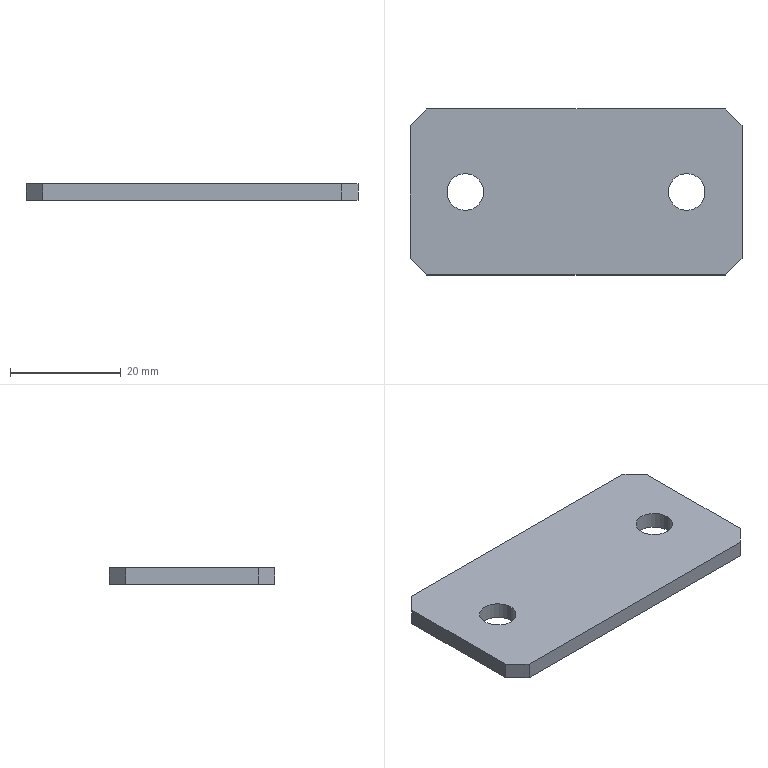Part | STEP file | HXGR200008-05-15 | 1 solid | 14 faces | box 60 x 30 x 3 mm | volume 5141 mm3 | plane 10 | cylinder 4 | commonest cylinder face diameters 6.6 x4
STEP:
#1=CARTESIAN_POINT('',(-23.3,0.,-3.));
#2=VERTEX_POINT('',#1);
#3=CARTESIAN_POINT('',(-16.7,0.,-3.));
#4=VERTEX_POINT('',#3);
#5=CARTESIAN_POINT('',(-20.,0.,-3.));
#6=DIRECTION('',(0.,0.,1.));
#7=DIRECTION('',(1.,0.,0.));
#8=AXIS2_PLACEMENT_3D('',#5,#6,#7);
#9=CIRCLE('',#8,3.3);
#10=EDGE_CURVE('',#2,#4,#9,.T.);
#11=ORIENTED_EDGE('',*,*,#10,.F.);
#12=CARTESIAN_POINT('',(-23.3,0.,0.));
#13=VERTEX_POINT('',#12);
#14=CARTESIAN_POINT('',(-23.3,0.,0.));
#15=DIRECTION('',(0.,0.,1.));
#16=VECTOR('',#15,1000.);
#17=LINE('',#14,#16);
#18=EDGE_CURVE('',#2,#13,#17,.T.);
#19=ORIENTED_EDGE('',*,*,#18,.T.);
#20=CARTESIAN_POINT('',(-16.7,0.,0.));
#21=VERTEX_POINT('',#20);
#22=CARTESIAN_POINT('',(-20.,0.,0.));
#23=DIRECTION('',(0.,0.,1.));
#24=DIRECTION('',(1.,0.,0.));
#25=AXIS2_PLACEMENT_3D('',#22,#23,#24);
#26=CIRCLE('',#25,3.3);
#27=EDGE_CURVE('',#13,#21,#26,.T.);
#28=ORIENTED_EDGE('',*,*,#27,.T.);
#29=CARTESIAN_POINT('',(-16.7,0.,0.));
#30=DIRECTION('',(0.,0.,1.));
#31=VECTOR('',#30,1000.);
#32=LINE('',#29,#31);
#33=EDGE_CURVE('',#4,#21,#32,.T.);
#34=ORIENTED_EDGE('',*,*,#33,.F.);
#35=EDGE_LOOP('',(#11,#19,#28,#34));
#36=FACE_OUTER_BOUND('',#35,.T.);
#37=CARTESIAN_POINT('',(-20.,0.,0.));
#38=DIRECTION('',(0.,0.,1.));
#39=DIRECTION('',(1.,0.,0.));
#40=AXIS2_PLACEMENT_3D('',#37,#38,#39);
#41=CYLINDRICAL_SURFACE('',#40,3.3);
#42=ADVANCED_FACE('',(#36),#41,.F.);
#43=CARTESIAN_POINT('',(16.7,0.,-3.));
#44=VERTEX_POINT('',#43);
#45=CARTESIAN_POINT('',(23.3,0.,-3.));
#46=VERTEX_POINT('',#45);
#47=CARTESIAN_POINT('',(20.,0.,-3.));
#48=DIRECTION('',(0.,0.,1.));
#49=DIRECTION('',(1.,0.,0.));
#50=AXIS2_PLACEMENT_3D('',#47,#48,#49);
#51=CIRCLE('',#50,3.3);
#52=EDGE_CURVE('',#44,#46,#51,.T.);
#53=ORIENTED_EDGE('',*,*,#52,.F.);
#54=CARTESIAN_POINT('',(16.7,0.,0.));
#55=VERTEX_POINT('',#54);
#56=CARTESIAN_POINT('',(16.7,0.,0.));
#57=DIRECTION('',(0.,0.,1.));
#58=VECTOR('',#57,1000.);
#59=LINE('',#56,#58);
#60=EDGE_CURVE('',#44,#55,#59,.T.);
#61=ORIENTED_EDGE('',*,*,#60,.T.);
#62=CARTESIAN_POINT('',(23.3,0.,0.));
#63=VERTEX_POINT('',#62);
#64=CARTESIAN_POINT('',(20.,0.,0.));
#65=DIRECTION('',(0.,0.,1.));
#66=DIRECTION('',(1.,0.,0.));
#67=AXIS2_PLACEMENT_3D('',#64,#65,#66);
#68=CIRCLE('',#67,3.3);
#69=EDGE_CURVE('',#55,#63,#68,.T.);
#70=ORIENTED_EDGE('',*,*,#69,.T.);
#71=CARTESIAN_POINT('',(23.3,0.,0.));
#72=DIRECTION('',(0.,0.,1.));
#73=VECTOR('',#72,1000.);
#74=LINE('',#71,#73);
#75=EDGE_CURVE('',#46,#63,#74,.T.);
#76=ORIENTED_EDGE('',*,*,#75,.F.);
#77=EDGE_LOOP('',(#53,#61,#70,#76));
#78=FACE_OUTER_BOUND('',#77,.T.);
#79=CARTESIAN_POINT('',(20.,0.,0.));
#80=DIRECTION('',(0.,0.,1.));
#81=DIRECTION('',(1.,0.,0.));
#82=AXIS2_PLACEMENT_3D('',#79,#80,#81);
#83=CYLINDRICAL_SURFACE('',#82,3.3);
#84=ADVANCED_FACE('',(#78),#83,.F.);
#85=CARTESIAN_POINT('',(30.,-12.,-3.));
#86=VERTEX_POINT('',#85);
#87=CARTESIAN_POINT('',(30.,12.,-3.));
#88=VERTEX_POINT('',#87);
#89=CARTESIAN_POINT('',(30.,15.,-3.));
#90=DIRECTION('',(0.,1.,0.));
#91=VECTOR('',#90,1000.);
#92=LINE('',#89,#91);
#93=EDGE_CURVE('',#86,#88,#92,.T.);
#94=ORIENTED_EDGE('',*,*,#93,.T.);
#95=CARTESIAN_POINT('',(30.,12.,0.));
#96=VERTEX_POINT('',#95);
#97=CARTESIAN_POINT('',(30.,12.,-3.));
#98=DIRECTION('',(0.,0.,1.));
#99=VECTOR('',#98,1000.);
#100=LINE('',#97,#99);
#101=EDGE_CURVE('',#88,#96,#100,.T.);
#102=ORIENTED_EDGE('',*,*,#101,.T.);
#103=CARTESIAN_POINT('',(30.,-12.,0.));
#104=VERTEX_POINT('',#103);
#105=CARTESIAN_POINT('',(30.,15.,0.));
#106=DIRECTION('',(0.,1.,0.));
#107=VECTOR('',#106,1000.);
#108=LINE('',#105,#107);
#109=EDGE_CURVE('',#104,#96,#108,.T.);
#110=ORIENTED_EDGE('',*,*,#109,.F.);
#111=CARTESIAN_POINT('',(30.,-12.,-3.));
#112=DIRECTION('',(0.,0.,-1.));
#113=VECTOR('',#112,1000.);
#114=LINE('',#111,#113);
#115=EDGE_CURVE('',#104,#86,#114,.T.);
#116=ORIENTED_EDGE('',*,*,#115,.T.);
#117=EDGE_LOOP('',(#94,#102,#110,#116));
#118=FACE_OUTER_BOUND('',#117,.T.);
#119=CARTESIAN_POINT('',(30.,15.,-3.));
#120=DIRECTION('',(1.,0.,0.));
#121=DIRECTION('',(0.,1.,0.));
#122=AXIS2_PLACEMENT_3D('',#119,#120,#121);
#123=PLANE('',#122);
#124=ADVANCED_FACE('',(#118),#123,.T.);
#125=CARTESIAN_POINT('',(-27.,-15.,-3.));
#126=VERTEX_POINT('',#125);
#127=CARTESIAN_POINT('',(27.,-15.,-3.));
#128=VERTEX_POINT('',#127);
#129=CARTESIAN_POINT('',(-30.,-15.,-3.));
#130=DIRECTION('',(1.,0.,0.));
#131=VECTOR('',#130,1000.);
#132=LINE('',#129,#131);
#133=EDGE_CURVE('',#126,#128,#132,.T.);
#134=ORIENTED_EDGE('',*,*,#133,.T.);
#135=CARTESIAN_POINT('',(27.,-15.,0.));
#136=VERTEX_POINT('',#135);
#137=CARTESIAN_POINT('',(27.,-15.,-3.));
#138=DIRECTION('',(0.,0.,1.));
#139=VECTOR('',#138,1000.);
#140=LINE('',#137,#139);
#141=EDGE_CURVE('',#128,#136,#140,.T.);
#142=ORIENTED_EDGE('',*,*,#141,.T.);
#143=CARTESIAN_POINT('',(-27.,-15.,0.));
#144=VERTEX_POINT('',#143);
#145=CARTESIAN_POINT('',(-30.,-15.,0.));
#146=DIRECTION('',(1.,0.,0.));
#147=VECTOR('',#146,1000.);
#148=LINE('',#145,#147);
#149=EDGE_CURVE('',#144,#136,#148,.T.);
#150=ORIENTED_EDGE('',*,*,#149,.F.);
#151=CARTESIAN_POINT('',(-27.,-15.,-3.));
#152=DIRECTION('',(0.,0.,-1.));
#153=VECTOR('',#152,1000.);
#154=LINE('',#151,#153);
#155=EDGE_CURVE('',#144,#126,#154,.T.);
#156=ORIENTED_EDGE('',*,*,#155,.T.);
#157=EDGE_LOOP('',(#134,#142,#150,#156));
#158=FACE_OUTER_BOUND('',#157,.T.);
#159=CARTESIAN_POINT('',(-30.,-15.,-3.));
#160=DIRECTION('',(0.,-1.,0.));
#161=DIRECTION('',(0.,0.,-1.));
#162=AXIS2_PLACEMENT_3D('',#159,#160,#161);
#163=PLANE('',#162);
#164=ADVANCED_FACE('',(#158),#163,.T.);
#165=CARTESIAN_POINT('',(-30.,12.,0.));
#166=VERTEX_POINT('',#165);
#167=CARTESIAN_POINT('',(-30.,-12.,0.));
#168=VERTEX_POINT('',#167);
#169=CARTESIAN_POINT('',(-30.,15.,0.));
#170=DIRECTION('',(0.,-1.,0.));
#171=VECTOR('',#170,1000.);
#172=LINE('',#169,#171);
#173=EDGE_CURVE('',#166,#168,#172,.T.);
#174=ORIENTED_EDGE('',*,*,#173,.F.);
#175=CARTESIAN_POINT('',(-30.,12.,-3.));
#176=VERTEX_POINT('',#175);
#177=CARTESIAN_POINT('',(-30.,12.,-3.));
#178=DIRECTION('',(0.,0.,-1.));
#179=VECTOR('',#178,1000.);
#180=LINE('',#177,#179);
#181=EDGE_CURVE('',#166,#176,#180,.T.);
#182=ORIENTED_EDGE('',*,*,#181,.T.);
#183=CARTESIAN_POINT('',(-30.,-12.,-3.));
#184=VERTEX_POINT('',#183);
#185=CARTESIAN_POINT('',(-30.,15.,-3.));
#186=DIRECTION('',(0.,-1.,0.));
#187=VECTOR('',#186,1000.);
#188=LINE('',#185,#187);
#189=EDGE_CURVE('',#176,#184,#188,.T.);
#190=ORIENTED_EDGE('',*,*,#189,.T.);
#191=CARTESIAN_POINT('',(-30.,-12.,-3.));
#192=DIRECTION('',(0.,0.,1.));
#193=VECTOR('',#192,1000.);
#194=LINE('',#191,#193);
#195=EDGE_CURVE('',#184,#168,#194,.T.);
#196=ORIENTED_EDGE('',*,*,#195,.T.);
#197=EDGE_LOOP('',(#174,#182,#190,#196));
#198=FACE_OUTER_BOUND('',#197,.T.);
#199=CARTESIAN_POINT('',(-30.,15.,-3.));
#200=DIRECTION('',(-1.,0.,0.));
#201=DIRECTION('',(0.,0.,1.));
#202=AXIS2_PLACEMENT_3D('',#199,#200,#201);
#203=PLANE('',#202);
#204=ADVANCED_FACE('',(#198),#203,.T.);
#205=CARTESIAN_POINT('',(27.,15.,-3.));
#206=VERTEX_POINT('',#205);
#207=CARTESIAN_POINT('',(-27.,15.,-3.));
#208=VERTEX_POINT('',#207);
#209=CARTESIAN_POINT('',(-30.,15.,-3.));
#210=DIRECTION('',(-1.,0.,0.));
#211=VECTOR('',#210,1000.);
#212=LINE('',#209,#211);
#213=EDGE_CURVE('',#206,#208,#212,.T.);
#214=ORIENTED_EDGE('',*,*,#213,.T.);
#215=CARTESIAN_POINT('',(-27.,15.,0.));
#216=VERTEX_POINT('',#215);
#217=CARTESIAN_POINT('',(-27.,15.,-3.));
#218=DIRECTION('',(0.,0.,1.));
#219=VECTOR('',#218,1000.);
#220=LINE('',#217,#219);
#221=EDGE_CURVE('',#208,#216,#220,.T.);
#222=ORIENTED_EDGE('',*,*,#221,.T.);
#223=CARTESIAN_POINT('',(27.,15.,0.));
#224=VERTEX_POINT('',#223);
#225=CARTESIAN_POINT('',(-30.,15.,0.));
#226=DIRECTION('',(-1.,0.,0.));
#227=VECTOR('',#226,1000.);
#228=LINE('',#225,#227);
#229=EDGE_CURVE('',#224,#216,#228,.T.);
#230=ORIENTED_EDGE('',*,*,#229,.F.);
#231=CARTESIAN_POINT('',(27.,15.,-3.));
#232=DIRECTION('',(0.,0.,-1.));
#233=VECTOR('',#232,1000.);
#234=LINE('',#231,#233);
#235=EDGE_CURVE('',#224,#206,#234,.T.);
#236=ORIENTED_EDGE('',*,*,#235,.T.);
#237=EDGE_LOOP('',(#214,#222,#230,#236));
#238=FACE_OUTER_BOUND('',#237,.T.);
#239=CARTESIAN_POINT('',(-30.,15.,-3.));
#240=DIRECTION('',(0.,1.,0.));
#241=DIRECTION('',(0.,0.,1.));
#242=AXIS2_PLACEMENT_3D('',#239,#240,#241);
#243=PLANE('',#242);
#244=ADVANCED_FACE('',(#238),#243,.T.);
#245=CARTESIAN_POINT('',(-20.,0.,-3.));
#246=DIRECTION('',(0.,0.,1.));
#247=DIRECTION('',(1.,0.,0.));
#248=AXIS2_PLACEMENT_3D('',#245,#246,#247);
#249=CIRCLE('',#248,3.3);
#250=EDGE_CURVE('',#4,#2,#249,.T.);
#251=ORIENTED_EDGE('',*,*,#250,.T.);
#252=ORIENTED_EDGE('',*,*,#10,.T.);
#253=EDGE_LOOP('',(#251,#252));
#254=FACE_BOUND('',#253,.T.);
#255=CARTESIAN_POINT('',(20.,0.,-3.));
#256=DIRECTION('',(0.,0.,1.));
#257=DIRECTION('',(1.,0.,0.));
#258=AXIS2_PLACEMENT_3D('',#255,#256,#257);
#259=CIRCLE('',#258,3.3);
#260=EDGE_CURVE('',#46,#44,#259,.T.);
#261=ORIENTED_EDGE('',*,*,#260,.T.);
#262=ORIENTED_EDGE('',*,*,#52,.T.);
#263=EDGE_LOOP('',(#261,#262));
#264=FACE_BOUND('',#263,.T.);
#265=ORIENTED_EDGE('',*,*,#189,.F.);
#266=CARTESIAN_POINT('',(-27.,15.,-3.));
#267=DIRECTION('',(0.7071,0.7071,0.));
#268=VECTOR('',#267,1000.);
#269=LINE('',#266,#268);
#270=EDGE_CURVE('',#176,#208,#269,.T.);
#271=ORIENTED_EDGE('',*,*,#270,.T.);
#272=ORIENTED_EDGE('',*,*,#213,.F.);
#273=CARTESIAN_POINT('',(30.,12.,-3.));
#274=DIRECTION('',(0.7071,-0.7071,0.));
#275=VECTOR('',#274,1000.);
#276=LINE('',#273,#275);
#277=EDGE_CURVE('',#206,#88,#276,.T.);
#278=ORIENTED_EDGE('',*,*,#277,.T.);
#279=ORIENTED_EDGE('',*,*,#93,.F.);
#280=CARTESIAN_POINT('',(27.,-15.,-3.));
#281=DIRECTION('',(-0.7071,-0.7071,0.));
#282=VECTOR('',#281,1000.);
#283=LINE('',#280,#282);
#284=EDGE_CURVE('',#86,#128,#283,.T.);
#285=ORIENTED_EDGE('',*,*,#284,.T.);
#286=ORIENTED_EDGE('',*,*,#133,.F.);
#287=CARTESIAN_POINT('',(-30.,-12.,-3.));
#288=DIRECTION('',(-0.7071,0.7071,0.));
#289=VECTOR('',#288,1000.);
#290=LINE('',#287,#289);
#291=EDGE_CURVE('',#126,#184,#290,.T.);
#292=ORIENTED_EDGE('',*,*,#291,.T.);
#293=EDGE_LOOP('',(#265,#271,#272,#278,#279,#285,#286,#292));
#294=FACE_OUTER_BOUND('',#293,.T.);
#295=CARTESIAN_POINT('',(0.,0.,-3.));
#296=DIRECTION('',(0.,0.,1.));
#297=DIRECTION('',(1.,0.,0.));
#298=AXIS2_PLACEMENT_3D('',#295,#296,#297);
#299=PLANE('',#298);
#300=ADVANCED_FACE('',(#254,#264,#294),#299,.F.);
#301=CARTESIAN_POINT('',(-20.,0.,0.));
#302=DIRECTION('',(0.,0.,1.));
#303=DIRECTION('',(1.,0.,0.));
#304=AXIS2_PLACEMENT_3D('',#301,#302,#303);
#305=CIRCLE('',#304,3.3);
#306=EDGE_CURVE('',#21,#13,#305,.T.);
#307=ORIENTED_EDGE('',*,*,#306,.F.);
#308=ORIENTED_EDGE('',*,*,#27,.F.);
#309=EDGE_LOOP('',(#307,#308));
#310=FACE_BOUND('',#309,.T.);
#311=CARTESIAN_POINT('',(20.,0.,0.));
#312=DIRECTION('',(0.,0.,1.));
#313=DIRECTION('',(1.,0.,0.));
#314=AXIS2_PLACEMENT_3D('',#311,#312,#313);
#315=CIRCLE('',#314,3.3);
#316=EDGE_CURVE('',#63,#55,#315,.T.);
#317=ORIENTED_EDGE('',*,*,#316,.F.);
#318=ORIENTED_EDGE('',*,*,#69,.F.);
#319=EDGE_LOOP('',(#317,#318));
#320=FACE_BOUND('',#319,.T.);
#321=ORIENTED_EDGE('',*,*,#229,.T.);
#322=CARTESIAN_POINT('',(-21.,21.,0.));
#323=DIRECTION('',(-0.7071,-0.7071,0.));
#324=VECTOR('',#323,1000.);
#325=LINE('',#322,#324);
#326=EDGE_CURVE('',#216,#166,#325,.T.);
#327=ORIENTED_EDGE('',*,*,#326,.T.);
#328=ORIENTED_EDGE('',*,*,#173,.T.);
#329=CARTESIAN_POINT('',(-21.,-21.,0.));
#330=DIRECTION('',(0.7071,-0.7071,0.));
#331=VECTOR('',#330,1000.);
#332=LINE('',#329,#331);
#333=EDGE_CURVE('',#168,#144,#332,.T.);
#334=ORIENTED_EDGE('',*,*,#333,.T.);
#335=ORIENTED_EDGE('',*,*,#149,.T.);
#336=CARTESIAN_POINT('',(21.,-21.,0.));
#337=DIRECTION('',(0.7071,0.7071,0.));
#338=VECTOR('',#337,1000.);
#339=LINE('',#336,#338);
#340=EDGE_CURVE('',#136,#104,#339,.T.);
#341=ORIENTED_EDGE('',*,*,#340,.T.);
#342=ORIENTED_EDGE('',*,*,#109,.T.);
#343=CARTESIAN_POINT('',(21.,21.,0.));
#344=DIRECTION('',(-0.7071,0.7071,0.));
#345=VECTOR('',#344,1000.);
#346=LINE('',#343,#345);
#347=EDGE_CURVE('',#96,#224,#346,.T.);
#348=ORIENTED_EDGE('',*,*,#347,.T.);
#349=EDGE_LOOP('',(#321,#327,#328,#334,#335,#341,#342,#348));
#350=FACE_OUTER_BOUND('',#349,.T.);
#351=CARTESIAN_POINT('',(0.,0.,0.));
#352=DIRECTION('',(0.,0.,1.));
#353=DIRECTION('',(1.,0.,0.));
#354=AXIS2_PLACEMENT_3D('',#351,#352,#353);
#355=PLANE('',#354);
#356=ADVANCED_FACE('',(#310,#320,#350),#355,.T.);
#357=ORIENTED_EDGE('',*,*,#270,.F.);
#358=ORIENTED_EDGE('',*,*,#181,.F.);
#359=ORIENTED_EDGE('',*,*,#326,.F.);
#360=ORIENTED_EDGE('',*,*,#221,.F.);
#361=EDGE_LOOP('',(#357,#358,#359,#360));
#362=FACE_OUTER_BOUND('',#361,.T.);
#363=CARTESIAN_POINT('',(-27.,15.,-3.));
#364=DIRECTION('',(0.7071,-0.7071,0.));
#365=DIRECTION('',(0.,0.,1.));
#366=AXIS2_PLACEMENT_3D('',#363,#364,#365);
#367=PLANE('',#366);
#368=ADVANCED_FACE('',(#362),#367,.F.);
#369=ORIENTED_EDGE('',*,*,#277,.F.);
#370=ORIENTED_EDGE('',*,*,#235,.F.);
#371=ORIENTED_EDGE('',*,*,#347,.F.);
#372=ORIENTED_EDGE('',*,*,#101,.F.);
#373=EDGE_LOOP('',(#369,#370,#371,#372));
#374=FACE_OUTER_BOUND('',#373,.T.);
#375=CARTESIAN_POINT('',(30.,12.,-3.));
#376=DIRECTION('',(-0.7071,-0.7071,0.));
#377=DIRECTION('',(0.,0.,1.));
#378=AXIS2_PLACEMENT_3D('',#375,#376,#377);
#379=PLANE('',#378);
#380=ADVANCED_FACE('',(#374),#379,.F.);
#381=ORIENTED_EDGE('',*,*,#284,.F.);
#382=ORIENTED_EDGE('',*,*,#115,.F.);
#383=ORIENTED_EDGE('',*,*,#340,.F.);
#384=ORIENTED_EDGE('',*,*,#141,.F.);
#385=EDGE_LOOP('',(#381,#382,#383,#384));
#386=FACE_OUTER_BOUND('',#385,.T.);
#387=CARTESIAN_POINT('',(27.,-15.,-3.));
#388=DIRECTION('',(-0.7071,0.7071,0.));
#389=DIRECTION('',(0.,0.,1.));
#390=AXIS2_PLACEMENT_3D('',#387,#388,#389);
#391=PLANE('',#390);
#392=ADVANCED_FACE('',(#386),#391,.F.);
#393=ORIENTED_EDGE('',*,*,#291,.F.);
#394=ORIENTED_EDGE('',*,*,#155,.F.);
#395=ORIENTED_EDGE('',*,*,#333,.F.);
#396=ORIENTED_EDGE('',*,*,#195,.F.);
#397=EDGE_LOOP('',(#393,#394,#395,#396));
#398=FACE_OUTER_BOUND('',#397,.T.);
#399=CARTESIAN_POINT('',(-30.,-12.,-3.));
#400=DIRECTION('',(0.7071,0.7071,0.));
#401=DIRECTION('',(0.,0.,1.));
#402=AXIS2_PLACEMENT_3D('',#399,#400,#401);
#403=PLANE('',#402);
#404=ADVANCED_FACE('',(#398),#403,.F.);
#405=ORIENTED_EDGE('',*,*,#60,.F.);
#406=ORIENTED_EDGE('',*,*,#260,.F.);
#407=ORIENTED_EDGE('',*,*,#75,.T.);
#408=ORIENTED_EDGE('',*,*,#316,.T.);
#409=EDGE_LOOP('',(#405,#406,#407,#408));
#410=FACE_OUTER_BOUND('',#409,.T.);
#411=CARTESIAN_POINT('',(20.,0.,0.));
#412=DIRECTION('',(0.,0.,1.));
#413=DIRECTION('',(1.,0.,0.));
#414=AXIS2_PLACEMENT_3D('',#411,#412,#413);
#415=CYLINDRICAL_SURFACE('',#414,3.3);
#416=ADVANCED_FACE('',(#410),#415,.F.);
#417=ORIENTED_EDGE('',*,*,#18,.F.);
#418=ORIENTED_EDGE('',*,*,#250,.F.);
#419=ORIENTED_EDGE('',*,*,#33,.T.);
#420=ORIENTED_EDGE('',*,*,#306,.T.);
#421=EDGE_LOOP('',(#417,#418,#419,#420));
#422=FACE_OUTER_BOUND('',#421,.T.);
#423=CARTESIAN_POINT('',(-20.,0.,0.));
#424=DIRECTION('',(0.,0.,1.));
#425=DIRECTION('',(1.,0.,0.));
#426=AXIS2_PLACEMENT_3D('',#423,#424,#425);
#427=CYLINDRICAL_SURFACE('',#426,3.3);
#428=ADVANCED_FACE('',(#422),#427,.F.);
#429=CLOSED_SHELL('',(#42,#84,#124,#164,#204,#244,#300,#356,#368,#380,#392,#404,#416,#428));
#430=MANIFOLD_SOLID_BREP('',#429);
#431=CARTESIAN_POINT('',(0.,0.,0.));
#432=DIRECTION('',(0.,0.,1.));
#433=DIRECTION('',(1.,0.,0.));
#434=AXIS2_PLACEMENT_3D('',#431,#432,#433);
#435=(LENGTH_UNIT()NAMED_UNIT(*)SI_UNIT(.MILLI.,.METRE.));
#436=UNCERTAINTY_MEASURE_WITH_UNIT(LENGTH_MEASURE(0.00001),#435,'','');
#437=(NAMED_UNIT(*)PLANE_ANGLE_UNIT()SI_UNIT($,.RADIAN.));
#438=(NAMED_UNIT(*)SI_UNIT($,.STERADIAN.)SOLID_ANGLE_UNIT());
#439=(GEOMETRIC_REPRESENTATION_CONTEXT(3)GLOBAL_UNCERTAINTY_ASSIGNED_CONTEXT((#436))GLOBAL_UNIT_ASSIGNED_CONTEXT((#435,#437,#438))REPRESENTATION_CONTEXT('',''));
#440=ADVANCED_BREP_SHAPE_REPRESENTATION('',(#430,#434),#439);